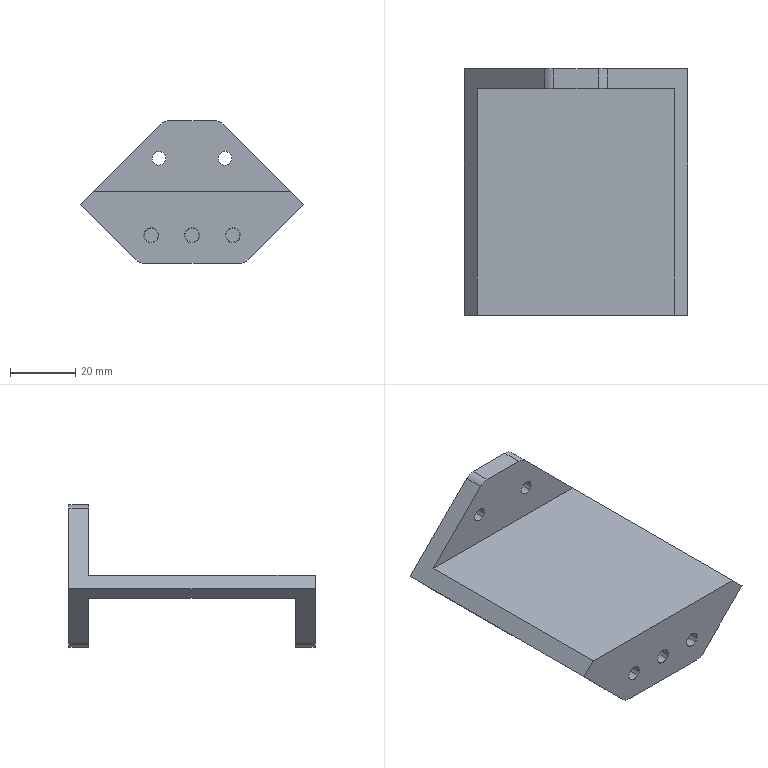NC program | NX | posted with a generic post | part box 68.307 x 75.3 x 43.668 mm
Lines 2877 to 2925 of 6865:
(FLOOR_WALL_1_COPY , TOOL : D10JING)
N5740 T14 M6
N5742 G54
N5744 G17 G0 G90 X38.153 Y-37.647 B0. C0. S9500 M3
N5746 G43 Z30. H14
N5748 Z-18.668
N5750 G94 G1 Z-21.668 F1250.
N5752 X35.153
N5754 X-35.153
N5756 Y-32.74
N5758 X35.153
N5760 Y-27.832
N5762 X-35.153
N5764 Y-22.925
N5766 X35.153
N5768 Y-18.017
N5770 X-35.153
N5772 Y-13.11
N5774 X35.153
N5776 Y-8.202
N5778 X-35.153
N5780 Y-3.295
N5782 X35.153
N5784 Y1.613
N5786 X-35.153
N5788 Y6.52
N5790 X35.153
N5792 Y11.428
N5794 X-35.153
N5796 Y16.335
N5798 X35.153
N5800 Y21.243
N5802 X-35.153
N5804 Y26.15
N5806 X35.153
N5808 X38.153
N5810 Z-18.668
N5812 G0 Z30.
N5814 Y26.65
N5816 Z-18.668
N5818 G1 Z-21.668
N5820 X35.153
N5822 X-35.153
N5824 X-38.153
N5826 Z-18.668
N5828 G0 Z30.
N5830 M5